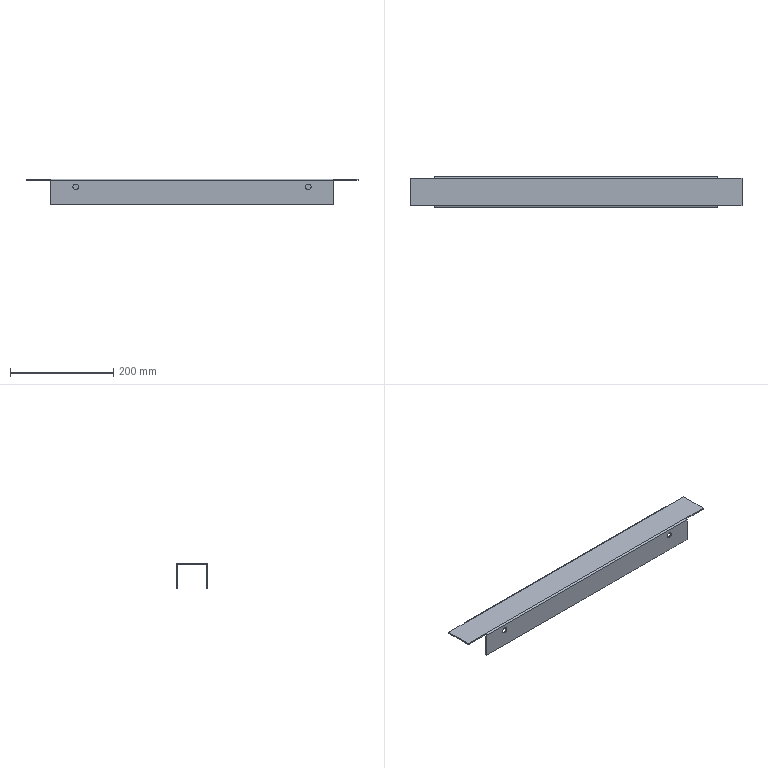Part | SolidWorks | features Cut 2, EdgeFlange 1, FlatPattern 1, ICE 1, MirrorPattern 1, SMBaseFlange 1, SheetMetal 1 | 1 solid | 34 faces | box 644 x 60 x 50 mm | volume 222593 mm3 | plane 22 | cylinder 12 | commonest cylinder face diameters 10.5 x4 11 x4 1 x2 6 x2
STEP:
#1=CARTESIAN_POINT('',(-225.5,-27.5,-9.5));
#2=VERTEX_POINT('',#1);
#3=CARTESIAN_POINT('',(-225.5,-27.5,-20.5));
#4=VERTEX_POINT('',#3);
#5=CARTESIAN_POINT('',(-225.5,-27.5,-15.));
#6=DIRECTION('',(0.,-1.,0.));
#7=DIRECTION('',(0.,0.,1.));
#8=AXIS2_PLACEMENT_3D('',#5,#6,#7);
#9=CIRCLE('',#8,5.5);
#10=EDGE_CURVE('',#2,#4,#9,.T.);
#11=ORIENTED_EDGE('',*,*,#10,.F.);
#12=CARTESIAN_POINT('',(-225.5,-30.,-9.5));
#13=VERTEX_POINT('',#12);
#14=CARTESIAN_POINT('',(-225.5,-20.,-9.5));
#15=DIRECTION('',(0.,-1.,0.));
#16=VECTOR('',#15,1000.);
#17=LINE('',#14,#16);
#18=EDGE_CURVE('',#2,#13,#17,.T.);
#19=ORIENTED_EDGE('',*,*,#18,.T.);
#20=CARTESIAN_POINT('',(-225.5,-30.,-20.5));
#21=VERTEX_POINT('',#20);
#22=CARTESIAN_POINT('',(-225.5,-30.,-15.));
#23=DIRECTION('',(0.,1.,0.));
#24=DIRECTION('',(0.,0.,-1.));
#25=AXIS2_PLACEMENT_3D('',#22,#23,#24);
#26=CIRCLE('',#25,5.5);
#27=EDGE_CURVE('',#21,#13,#26,.T.);
#28=ORIENTED_EDGE('',*,*,#27,.F.);
#29=CARTESIAN_POINT('',(-225.5,-20.,-20.5));
#30=DIRECTION('',(0.,-1.,0.));
#31=VECTOR('',#30,1000.);
#32=LINE('',#29,#31);
#33=EDGE_CURVE('',#4,#21,#32,.T.);
#34=ORIENTED_EDGE('',*,*,#33,.F.);
#35=EDGE_LOOP('',(#11,#19,#28,#34));
#36=FACE_OUTER_BOUND('',#35,.T.);
#37=CARTESIAN_POINT('',(-225.5,-20.,-15.));
#38=DIRECTION('',(0.,-1.,0.));
#39=DIRECTION('',(0.,0.,-1.));
#40=AXIS2_PLACEMENT_3D('',#37,#38,#39);
#41=CYLINDRICAL_SURFACE('',#40,5.5);
#42=ADVANCED_FACE('',(#36),#41,.F.);
#43=CARTESIAN_POINT('',(225.5,-27.5,-20.5));
#44=VERTEX_POINT('',#43);
#45=CARTESIAN_POINT('',(225.5,-27.5,-9.5));
#46=VERTEX_POINT('',#45);
#47=CARTESIAN_POINT('',(225.5,-27.5,-15.));
#48=DIRECTION('',(0.,1.,0.));
#49=DIRECTION('',(0.,0.,1.));
#50=AXIS2_PLACEMENT_3D('',#47,#48,#49);
#51=CIRCLE('',#50,5.5);
#52=EDGE_CURVE('',#44,#46,#51,.T.);
#53=ORIENTED_EDGE('',*,*,#52,.T.);
#54=CARTESIAN_POINT('',(225.5,-30.,-9.5));
#55=VERTEX_POINT('',#54);
#56=CARTESIAN_POINT('',(225.5,-20.,-9.5));
#57=DIRECTION('',(0.,-1.,0.));
#58=VECTOR('',#57,1000.);
#59=LINE('',#56,#58);
#60=EDGE_CURVE('',#46,#55,#59,.T.);
#61=ORIENTED_EDGE('',*,*,#60,.T.);
#62=CARTESIAN_POINT('',(225.5,-30.,-20.5));
#63=VERTEX_POINT('',#62);
#64=CARTESIAN_POINT('',(225.5,-30.,-15.));
#65=DIRECTION('',(0.,-1.,0.));
#66=DIRECTION('',(0.,0.,-1.));
#67=AXIS2_PLACEMENT_3D('',#64,#65,#66);
#68=CIRCLE('',#67,5.5);
#69=EDGE_CURVE('',#55,#63,#68,.T.);
#70=ORIENTED_EDGE('',*,*,#69,.T.);
#71=CARTESIAN_POINT('',(225.5,-20.,-20.5));
#72=DIRECTION('',(0.,-1.,0.));
#73=VECTOR('',#72,1000.);
#74=LINE('',#71,#73);
#75=EDGE_CURVE('',#44,#63,#74,.T.);
#76=ORIENTED_EDGE('',*,*,#75,.F.);
#77=EDGE_LOOP('',(#53,#61,#70,#76));
#78=FACE_OUTER_BOUND('',#77,.T.);
#79=CARTESIAN_POINT('',(225.5,-20.,-15.));
#80=DIRECTION('',(0.,-1.,0.));
#81=DIRECTION('',(0.,0.,-1.));
#82=AXIS2_PLACEMENT_3D('',#79,#80,#81);
#83=CYLINDRICAL_SURFACE('',#82,5.5);
#84=ADVANCED_FACE('',(#78),#83,.F.);
#85=CARTESIAN_POINT('',(225.,27.5,-30.25));
#86=VERTEX_POINT('',#85);
#87=CARTESIAN_POINT('',(225.,27.5,-19.75));
#88=VERTEX_POINT('',#87);
#89=CARTESIAN_POINT('',(225.,27.5,-25.));
#90=DIRECTION('',(0.,1.,0.));
#91=DIRECTION('',(0.,0.,1.));
#92=AXIS2_PLACEMENT_3D('',#89,#90,#91);
#93=CIRCLE('',#92,5.25);
#94=EDGE_CURVE('',#86,#88,#93,.T.);
#95=ORIENTED_EDGE('',*,*,#94,.F.);
#96=CARTESIAN_POINT('',(225.,30.,-30.25));
#97=VERTEX_POINT('',#96);
#98=CARTESIAN_POINT('',(225.,20.,-30.25));
#99=DIRECTION('',(0.,1.,0.));
#100=VECTOR('',#99,1000.);
#101=LINE('',#98,#100);
#102=EDGE_CURVE('',#86,#97,#101,.T.);
#103=ORIENTED_EDGE('',*,*,#102,.T.);
#104=CARTESIAN_POINT('',(225.,30.,-19.75));
#105=VERTEX_POINT('',#104);
#106=CARTESIAN_POINT('',(225.,30.,-25.));
#107=DIRECTION('',(0.,1.,0.));
#108=DIRECTION('',(0.,0.,-1.));
#109=AXIS2_PLACEMENT_3D('',#106,#107,#108);
#110=CIRCLE('',#109,5.25);
#111=EDGE_CURVE('',#97,#105,#110,.T.);
#112=ORIENTED_EDGE('',*,*,#111,.T.);
#113=CARTESIAN_POINT('',(225.,20.,-19.75));
#114=DIRECTION('',(0.,1.,0.));
#115=VECTOR('',#114,1000.);
#116=LINE('',#113,#115);
#117=EDGE_CURVE('',#88,#105,#116,.T.);
#118=ORIENTED_EDGE('',*,*,#117,.F.);
#119=EDGE_LOOP('',(#95,#103,#112,#118));
#120=FACE_OUTER_BOUND('',#119,.T.);
#121=CARTESIAN_POINT('',(225.,20.,-25.));
#122=DIRECTION('',(0.,1.,0.));
#123=DIRECTION('',(0.,0.,1.));
#124=AXIS2_PLACEMENT_3D('',#121,#122,#123);
#125=CYLINDRICAL_SURFACE('',#124,5.25);
#126=ADVANCED_FACE('',(#120),#125,.F.);
#127=CARTESIAN_POINT('',(-225.,27.5,-30.25));
#128=VERTEX_POINT('',#127);
#129=CARTESIAN_POINT('',(-225.,27.5,-19.75));
#130=VERTEX_POINT('',#129);
#131=CARTESIAN_POINT('',(-225.,27.5,-25.));
#132=DIRECTION('',(0.,1.,0.));
#133=DIRECTION('',(0.,0.,1.));
#134=AXIS2_PLACEMENT_3D('',#131,#132,#133);
#135=CIRCLE('',#134,5.25);
#136=EDGE_CURVE('',#128,#130,#135,.T.);
#137=ORIENTED_EDGE('',*,*,#136,.F.);
#138=CARTESIAN_POINT('',(-225.,30.,-30.25));
#139=VERTEX_POINT('',#138);
#140=CARTESIAN_POINT('',(-225.,20.,-30.25));
#141=DIRECTION('',(0.,1.,0.));
#142=VECTOR('',#141,1000.);
#143=LINE('',#140,#142);
#144=EDGE_CURVE('',#128,#139,#143,.T.);
#145=ORIENTED_EDGE('',*,*,#144,.T.);
#146=CARTESIAN_POINT('',(-225.,30.,-19.75));
#147=VERTEX_POINT('',#146);
#148=CARTESIAN_POINT('',(-225.,30.,-25.));
#149=DIRECTION('',(0.,1.,0.));
#150=DIRECTION('',(0.,0.,1.));
#151=AXIS2_PLACEMENT_3D('',#148,#149,#150);
#152=CIRCLE('',#151,5.25);
#153=EDGE_CURVE('',#139,#147,#152,.T.);
#154=ORIENTED_EDGE('',*,*,#153,.T.);
#155=CARTESIAN_POINT('',(-225.,20.,-19.75));
#156=DIRECTION('',(0.,1.,0.));
#157=VECTOR('',#156,1000.);
#158=LINE('',#155,#157);
#159=EDGE_CURVE('',#130,#147,#158,.T.);
#160=ORIENTED_EDGE('',*,*,#159,.F.);
#161=EDGE_LOOP('',(#137,#145,#154,#160));
#162=FACE_OUTER_BOUND('',#161,.T.);
#163=CARTESIAN_POINT('',(-225.,20.,-25.));
#164=DIRECTION('',(0.,1.,0.));
#165=DIRECTION('',(0.,0.,1.));
#166=AXIS2_PLACEMENT_3D('',#163,#164,#165);
#167=CYLINDRICAL_SURFACE('',#166,5.25);
#168=ADVANCED_FACE('',(#162),#167,.F.);
#169=CARTESIAN_POINT('',(-274.5,-30.,-3.));
#170=VERTEX_POINT('',#169);
#171=CARTESIAN_POINT('',(274.5,-30.,-3.));
#172=VERTEX_POINT('',#171);
#173=CARTESIAN_POINT('',(274.5,-30.,-3.));
#174=DIRECTION('',(1.,0.,0.));
#175=VECTOR('',#174,1000.);
#176=LINE('',#173,#175);
#177=EDGE_CURVE('',#170,#172,#176,.T.);
#178=ORIENTED_EDGE('',*,*,#177,.F.);
#179=CARTESIAN_POINT('',(-274.5,-30.,-50.));
#180=VERTEX_POINT('',#179);
#181=CARTESIAN_POINT('',(-274.5,-30.,-50.));
#182=DIRECTION('',(0.,0.,1.));
#183=VECTOR('',#182,1000.);
#184=LINE('',#181,#183);
#185=EDGE_CURVE('',#180,#170,#184,.T.);
#186=ORIENTED_EDGE('',*,*,#185,.F.);
#187=CARTESIAN_POINT('',(274.5,-30.,-50.));
#188=VERTEX_POINT('',#187);
#189=CARTESIAN_POINT('',(274.5,-30.,-50.));
#190=DIRECTION('',(-1.,0.,0.));
#191=VECTOR('',#190,1000.);
#192=LINE('',#189,#191);
#193=EDGE_CURVE('',#188,#180,#192,.T.);
#194=ORIENTED_EDGE('',*,*,#193,.F.);
#195=CARTESIAN_POINT('',(274.5,-30.,-2.5));
#196=DIRECTION('',(0.,0.,-1.));
#197=VECTOR('',#196,1000.);
#198=LINE('',#195,#197);
#199=EDGE_CURVE('',#172,#188,#198,.T.);
#200=ORIENTED_EDGE('',*,*,#199,.F.);
#201=EDGE_LOOP('',(#178,#186,#194,#200));
#202=FACE_OUTER_BOUND('',#201,.T.);
#203=CARTESIAN_POINT('',(225.5,-30.,-15.));
#204=DIRECTION('',(0.,-1.,0.));
#205=DIRECTION('',(0.,0.,-1.));
#206=AXIS2_PLACEMENT_3D('',#203,#204,#205);
#207=CIRCLE('',#206,5.5);
#208=EDGE_CURVE('',#63,#55,#207,.T.);
#209=ORIENTED_EDGE('',*,*,#208,.F.);
#210=ORIENTED_EDGE('',*,*,#69,.F.);
#211=EDGE_LOOP('',(#209,#210));
#212=FACE_BOUND('',#211,.T.);
#213=ORIENTED_EDGE('',*,*,#27,.T.);
#214=CARTESIAN_POINT('',(-225.5,-30.,-15.));
#215=DIRECTION('',(0.,1.,0.));
#216=DIRECTION('',(0.,0.,-1.));
#217=AXIS2_PLACEMENT_3D('',#214,#215,#216);
#218=CIRCLE('',#217,5.5);
#219=EDGE_CURVE('',#13,#21,#218,.T.);
#220=ORIENTED_EDGE('',*,*,#219,.T.);
#221=EDGE_LOOP('',(#213,#220));
#222=FACE_BOUND('',#221,.T.);
#223=CARTESIAN_POINT('',(0.,-30.,0.));
#224=DIRECTION('',(0.,1.,0.));
#225=DIRECTION('',(0.,0.,1.));
#226=AXIS2_PLACEMENT_3D('',#223,#224,#225);
#227=PLANE('',#226);
#228=ADVANCED_FACE('',(#202,#212,#222),#227,.F.);
#229=CARTESIAN_POINT('',(-274.5,-27.5,-50.));
#230=VERTEX_POINT('',#229);
#231=CARTESIAN_POINT('',(-274.5,-27.5,-3.));
#232=VERTEX_POINT('',#231);
#233=CARTESIAN_POINT('',(-274.5,-27.5,0.));
#234=DIRECTION('',(0.,0.,1.));
#235=VECTOR('',#234,1000.);
#236=LINE('',#233,#235);
#237=EDGE_CURVE('',#230,#232,#236,.T.);
#238=ORIENTED_EDGE('',*,*,#237,.T.);
#239=CARTESIAN_POINT('',(274.5,-27.5,-3.));
#240=VERTEX_POINT('',#239);
#241=CARTESIAN_POINT('',(274.5,-27.5,-3.));
#242=DIRECTION('',(-1.,0.,0.));
#243=VECTOR('',#242,1000.);
#244=LINE('',#241,#243);
#245=EDGE_CURVE('',#240,#232,#244,.T.);
#246=ORIENTED_EDGE('',*,*,#245,.F.);
#247=CARTESIAN_POINT('',(274.5,-27.5,-50.));
#248=VERTEX_POINT('',#247);
#249=CARTESIAN_POINT('',(274.5,-27.5,0.));
#250=DIRECTION('',(0.,0.,-1.));
#251=VECTOR('',#250,1000.);
#252=LINE('',#249,#251);
#253=EDGE_CURVE('',#240,#248,#252,.T.);
#254=ORIENTED_EDGE('',*,*,#253,.T.);
#255=CARTESIAN_POINT('',(0.,-27.5,-50.));
#256=DIRECTION('',(-1.,0.,0.));
#257=VECTOR('',#256,1000.);
#258=LINE('',#255,#257);
#259=EDGE_CURVE('',#248,#230,#258,.T.);
#260=ORIENTED_EDGE('',*,*,#259,.T.);
#261=EDGE_LOOP('',(#238,#246,#254,#260));
#262=FACE_OUTER_BOUND('',#261,.T.);
#263=ORIENTED_EDGE('',*,*,#52,.F.);
#264=CARTESIAN_POINT('',(225.5,-27.5,-15.));
#265=DIRECTION('',(0.,1.,0.));
#266=DIRECTION('',(0.,0.,1.));
#267=AXIS2_PLACEMENT_3D('',#264,#265,#266);
#268=CIRCLE('',#267,5.5);
#269=EDGE_CURVE('',#46,#44,#268,.T.);
#270=ORIENTED_EDGE('',*,*,#269,.F.);
#271=EDGE_LOOP('',(#263,#270));
#272=FACE_BOUND('',#271,.T.);
#273=CARTESIAN_POINT('',(-225.5,-27.5,-15.));
#274=DIRECTION('',(0.,-1.,0.));
#275=DIRECTION('',(0.,0.,1.));
#276=AXIS2_PLACEMENT_3D('',#273,#274,#275);
#277=CIRCLE('',#276,5.5);
#278=EDGE_CURVE('',#4,#2,#277,.T.);
#279=ORIENTED_EDGE('',*,*,#278,.T.);
#280=ORIENTED_EDGE('',*,*,#10,.T.);
#281=EDGE_LOOP('',(#279,#280));
#282=FACE_BOUND('',#281,.T.);
#283=CARTESIAN_POINT('',(0.,-27.5,0.));
#284=DIRECTION('',(0.,1.,0.));
#285=DIRECTION('',(0.,0.,1.));
#286=AXIS2_PLACEMENT_3D('',#283,#284,#285);
#287=PLANE('',#286);
#288=ADVANCED_FACE('',(#262,#272,#282),#287,.T.);
#289=CARTESIAN_POINT('',(-322.,-27.,-2.5));
#290=VERTEX_POINT('',#289);
#291=CARTESIAN_POINT('',(-274.5,-27.,-2.5));
#292=VERTEX_POINT('',#291);
#293=CARTESIAN_POINT('',(-322.,-27.,-2.5));
#294=DIRECTION('',(1.,0.,0.));
#295=VECTOR('',#294,1000.);
#296=LINE('',#293,#295);
#297=EDGE_CURVE('',#290,#292,#296,.T.);
#298=ORIENTED_EDGE('',*,*,#297,.T.);
#299=CARTESIAN_POINT('',(-274.5,-27.,0.));
#300=VERTEX_POINT('',#299);
#301=CARTESIAN_POINT('',(-274.5,-27.,-2.5));
#302=DIRECTION('',(0.,0.,1.));
#303=VECTOR('',#302,1000.);
#304=LINE('',#301,#303);
#305=EDGE_CURVE('',#292,#300,#304,.T.);
#306=ORIENTED_EDGE('',*,*,#305,.T.);
#307=CARTESIAN_POINT('',(-322.,-27.,0.));
#308=VERTEX_POINT('',#307);
#309=CARTESIAN_POINT('',(-322.,-27.,0.));
#310=DIRECTION('',(1.,0.,0.));
#311=VECTOR('',#310,1000.);
#312=LINE('',#309,#311);
#313=EDGE_CURVE('',#308,#300,#312,.T.);
#314=ORIENTED_EDGE('',*,*,#313,.F.);
#315=CARTESIAN_POINT('',(-322.,-27.,-2.5));
#316=DIRECTION('',(0.,0.,1.));
#317=VECTOR('',#316,1000.);
#318=LINE('',#315,#317);
#319=EDGE_CURVE('',#290,#308,#318,.T.);
#320=ORIENTED_EDGE('',*,*,#319,.F.);
#321=EDGE_LOOP('',(#298,#306,#314,#320));
#322=FACE_OUTER_BOUND('',#321,.T.);
#323=CARTESIAN_POINT('',(-322.,-27.,-2.5));
#324=DIRECTION('',(0.,-1.,0.));
#325=DIRECTION('',(0.,0.,-1.));
#326=AXIS2_PLACEMENT_3D('',#323,#324,#325);
#327=PLANE('',#326);
#328=ADVANCED_FACE('',(#322),#327,.T.);
#329=CARTESIAN_POINT('',(322.,27.,-2.5));
#330=VERTEX_POINT('',#329);
#331=CARTESIAN_POINT('',(274.5,27.,-2.5));
#332=VERTEX_POINT('',#331);
#333=CARTESIAN_POINT('',(-322.,27.,-2.5));
#334=DIRECTION('',(-1.,0.,0.));
#335=VECTOR('',#334,1000.);
#336=LINE('',#333,#335);
#337=EDGE_CURVE('',#330,#332,#336,.T.);
#338=ORIENTED_EDGE('',*,*,#337,.T.);
#339=CARTESIAN_POINT('',(274.5,27.,0.));
#340=VERTEX_POINT('',#339);
#341=CARTESIAN_POINT('',(274.5,27.,-2.5));
#342=DIRECTION('',(0.,0.,1.));
#343=VECTOR('',#342,1000.);
#344=LINE('',#341,#343);
#345=EDGE_CURVE('',#332,#340,#344,.T.);
#346=ORIENTED_EDGE('',*,*,#345,.T.);
#347=CARTESIAN_POINT('',(322.,27.,0.));
#348=VERTEX_POINT('',#347);
#349=CARTESIAN_POINT('',(-322.,27.,0.));
#350=DIRECTION('',(-1.,0.,0.));
#351=VECTOR('',#350,1000.);
#352=LINE('',#349,#351);
#353=EDGE_CURVE('',#348,#340,#352,.T.);
#354=ORIENTED_EDGE('',*,*,#353,.F.);
#355=CARTESIAN_POINT('',(322.,27.,-2.5));
#356=DIRECTION('',(0.,0.,1.));
#357=VECTOR('',#356,1000.);
#358=LINE('',#355,#357);
#359=EDGE_CURVE('',#330,#348,#358,.T.);
#360=ORIENTED_EDGE('',*,*,#359,.F.);
#361=EDGE_LOOP('',(#338,#346,#354,#360));
#362=FACE_OUTER_BOUND('',#361,.T.);
#363=CARTESIAN_POINT('',(-322.,27.,-2.5));
#364=DIRECTION('',(0.,1.,0.));
#365=DIRECTION('',(0.,0.,1.));
#366=AXIS2_PLACEMENT_3D('',#363,#364,#365);
#367=PLANE('',#366);
#368=ADVANCED_FACE('',(#362),#367,.T.);
#369=CARTESIAN_POINT('',(322.,-27.,0.));
#370=VERTEX_POINT('',#369);
#371=CARTESIAN_POINT('',(322.,27.,0.));
#372=DIRECTION('',(0.,1.,0.));
#373=VECTOR('',#372,1000.);
#374=LINE('',#371,#373);
#375=EDGE_CURVE('',#370,#348,#374,.T.);
#376=ORIENTED_EDGE('',*,*,#375,.F.);
#377=CARTESIAN_POINT('',(322.,-27.,-2.5));
#378=VERTEX_POINT('',#377);
#379=CARTESIAN_POINT('',(322.,-27.,-2.5));
#380=DIRECTION('',(0.,0.,1.));
#381=VECTOR('',#380,1000.);
#382=LINE('',#379,#381);
#383=EDGE_CURVE('',#378,#370,#382,.T.);
#384=ORIENTED_EDGE('',*,*,#383,.F.);
#385=CARTESIAN_POINT('',(322.,27.,-2.5));
#386=DIRECTION('',(0.,1.,0.));
#387=VECTOR('',#386,1000.);
#388=LINE('',#385,#387);
#389=EDGE_CURVE('',#378,#330,#388,.T.);
#390=ORIENTED_EDGE('',*,*,#389,.T.);
#391=ORIENTED_EDGE('',*,*,#359,.T.);
#392=EDGE_LOOP('',(#376,#384,#390,#391));
#393=FACE_OUTER_BOUND('',#392,.T.);
#394=CARTESIAN_POINT('',(322.,27.,-2.5));
#395=DIRECTION('',(1.,0.,0.));
#396=DIRECTION('',(0.,0.,-1.));
#397=AXIS2_PLACEMENT_3D('',#394,#395,#396);
#398=PLANE('',#397);
#399=ADVANCED_FACE('',(#393),#398,.T.);
#400=CARTESIAN_POINT('',(274.5,-27.,-2.5));
#401=VERTEX_POINT('',#400);
#402=CARTESIAN_POINT('',(274.5,-27.,0.));
#403=VERTEX_POINT('',#402);
#404=CARTESIAN_POINT('',(274.5,-27.,-2.5));
#405=DIRECTION('',(0.,0.,1.));
#406=VECTOR('',#405,1000.);
#407=LINE('',#404,#406);
#408=EDGE_CURVE('',#401,#403,#407,.T.);
#409=ORIENTED_EDGE('',*,*,#408,.F.);
#410=CARTESIAN_POINT('',(-322.,-27.,-2.5));
#411=DIRECTION('',(1.,0.,0.));
#412=VECTOR('',#411,1000.);
#413=LINE('',#410,#412);
#414=EDGE_CURVE('',#401,#378,#413,.T.);
#415=ORIENTED_EDGE('',*,*,#414,.T.);
#416=ORIENTED_EDGE('',*,*,#383,.T.);
#417=CARTESIAN_POINT('',(-322.,-27.,0.));
#418=DIRECTION('',(1.,0.,0.));
#419=VECTOR('',#418,1000.);
#420=LINE('',#417,#419);
#421=EDGE_CURVE('',#403,#370,#420,.T.);
#422=ORIENTED_EDGE('',*,*,#421,.F.);
#423=EDGE_LOOP('',(#409,#415,#416,#422));
#424=FACE_OUTER_BOUND('',#423,.T.);
#425=CARTESIAN_POINT('',(-322.,-27.,-2.5));
#426=DIRECTION('',(0.,-1.,0.));
#427=DIRECTION('',(0.,0.,-1.));
#428=AXIS2_PLACEMENT_3D('',#425,#426,#427);
#429=PLANE('',#428);
#430=ADVANCED_FACE('',(#424),#429,.T.);
#431=CARTESIAN_POINT('',(-322.,27.,0.));
#432=VERTEX_POINT('',#431);
#433=CARTESIAN_POINT('',(-322.,27.,0.));
#434=DIRECTION('',(0.,-1.,0.));
#435=VECTOR('',#434,1000.);
#436=LINE('',#433,#435);
#437=EDGE_CURVE('',#432,#308,#436,.T.);
#438=ORIENTED_EDGE('',*,*,#437,.F.);
#439=CARTESIAN_POINT('',(-322.,27.,-2.5));
#440=VERTEX_POINT('',#439);
#441=CARTESIAN_POINT('',(-322.,27.,-2.5));
#442=DIRECTION('',(0.,0.,1.));
#443=VECTOR('',#442,1000.);
#444=LINE('',#441,#443);
#445=EDGE_CURVE('',#440,#432,#444,.T.);
#446=ORIENTED_EDGE('',*,*,#445,.F.);
#447=CARTESIAN_POINT('',(-322.,27.,-2.5));
#448=DIRECTION('',(0.,-1.,0.));
#449=VECTOR('',#448,1000.);
#450=LINE('',#447,#449);
#451=EDGE_CURVE('',#440,#290,#450,.T.);
#452=ORIENTED_EDGE('',*,*,#451,.T.);
#453=ORIENTED_EDGE('',*,*,#319,.T.);
#454=EDGE_LOOP('',(#438,#446,#452,#453));
#455=FACE_OUTER_BOUND('',#454,.T.);
#456=CARTESIAN_POINT('',(-322.,27.,-2.5));
#457=DIRECTION('',(-1.,0.,0.));
#458=DIRECTION('',(0.,0.,1.));
#459=AXIS2_PLACEMENT_3D('',#456,#457,#458);
#460=PLANE('',#459);
#461=ADVANCED_FACE('',(#455),#460,.T.);
#462=CARTESIAN_POINT('',(-274.5,27.,-2.5));
#463=VERTEX_POINT('',#462);
#464=CARTESIAN_POINT('',(-274.5,27.,0.));
#465=VERTEX_POINT('',#464);
#466=CARTESIAN_POINT('',(-274.5,27.,-2.5));
#467=DIRECTION('',(0.,0.,1.));
#468=VECTOR('',#467,1000.);
#469=LINE('',#466,#468);
#470=EDGE_CURVE('',#463,#465,#469,.T.);
#471=ORIENTED_EDGE('',*,*,#470,.F.);
#472=CARTESIAN_POINT('',(-322.,27.,-2.5));
#473=DIRECTION('',(-1.,0.,0.));
#474=VECTOR('',#473,1000.);
#475=LINE('',#472,#474);
#476=EDGE_CURVE('',#463,#440,#475,.T.);
#477=ORIENTED_EDGE('',*,*,#476,.T.);
#478=ORIENTED_EDGE('',*,*,#445,.T.);
#479=CARTESIAN_POINT('',(-322.,27.,0.));
#480=DIRECTION('',(-1.,0.,0.));
#481=VECTOR('',#480,1000.);
#482=LINE('',#479,#481);
#483=EDGE_CURVE('',#465,#432,#482,.T.);
#484=ORIENTED_EDGE('',*,*,#483,.F.);
#485=EDGE_LOOP('',(#471,#477,#478,#484));
#486=FACE_OUTER_BOUND('',#485,.T.);
#487=CARTESIAN_POINT('',(-322.,27.,-2.5));
#488=DIRECTION('',(0.,1.,0.));
#489=DIRECTION('',(0.,0.,1.));
#490=AXIS2_PLACEMENT_3D('',#487,#488,#489);
#491=PLANE('',#490);
#492=ADVANCED_FACE('',(#486),#491,.T.);
#493=ORIENTED_EDGE('',*,*,#389,.F.);
#494=ORIENTED_EDGE('',*,*,#414,.F.);
#495=CARTESIAN_POINT('',(-274.5,-27.,-2.5));
#496=DIRECTION('',(1.,0.,0.));
#497=VECTOR('',#496,1000.);
#498=LINE('',#495,#497);
#499=EDGE_CURVE('',#292,#401,#498,.T.);
#500=ORIENTED_EDGE('',*,*,#499,.F.);
#501=ORIENTED_EDGE('',*,*,#297,.F.);
#502=ORIENTED_EDGE('',*,*,#451,.F.);
#503=ORIENTED_EDGE('',*,*,#476,.F.);
#504=CARTESIAN_POINT('',(274.5,27.,-2.5));
#505=DIRECTION('',(-1.,0.,0.));
#506=VECTOR('',#505,1000.);
#507=LINE('',#504,#506);
#508=EDGE_CURVE('',#332,#463,#507,.T.);
#509=ORIENTED_EDGE('',*,*,#508,.F.);
#510=ORIENTED_EDGE('',*,*,#337,.F.);
#511=EDGE_LOOP('',(#493,#494,#500,#501,#502,#503,#509,#510));
#512=FACE_OUTER_BOUND('',#511,.T.);
#513=CARTESIAN_POINT('',(0.,0.,-2.5));
#514=DIRECTION('',(0.,0.,1.));
#515=DIRECTION('',(1.,0.,0.));
#516=AXIS2_PLACEMENT_3D('',#513,#514,#515);
#517=PLANE('',#516);
#518=ADVANCED_FACE('',(#512),#517,.F.);
#519=ORIENTED_EDGE('',*,*,#375,.T.);
#520=ORIENTED_EDGE('',*,*,#353,.T.);
#521=CARTESIAN_POINT('',(274.5,27.,0.));
#522=DIRECTION('',(-1.,0.,0.));
#523=VECTOR('',#522,1000.);
#524=LINE('',#521,#523);
#525=EDGE_CURVE('',#340,#465,#524,.T.);
#526=ORIENTED_EDGE('',*,*,#525,.T.);
#527=ORIENTED_EDGE('',*,*,#483,.T.);
#528=ORIENTED_EDGE('',*,*,#437,.T.);
#529=ORIENTED_EDGE('',*,*,#313,.T.);
#530=CARTESIAN_POINT('',(-274.5,-27.,0.));
#531=DIRECTION('',(1.,0.,0.));
#532=VECTOR('',#531,1000.);
#533=LINE('',#530,#532);
#534=EDGE_CURVE('',#300,#403,#533,.T.);
#535=ORIENTED_EDGE('',*,*,#534,.T.);
#536=ORIENTED_EDGE('',*,*,#421,.T.);
#537=EDGE_LOOP('',(#519,#520,#526,#527,#528,#529,#535,#536));
#538=FACE_OUTER_BOUND('',#537,.T.);
#539=CARTESIAN_POINT('',(0.,0.,0.));
#540=DIRECTION('',(0.,0.,1.));
#541=DIRECTION('',(1.,0.,0.));
#542=AXIS2_PLACEMENT_3D('',#539,#540,#541);
#543=PLANE('',#542);
#544=ADVANCED_FACE('',(#538),#543,.T.);
#545=CARTESIAN_POINT('',(-274.5,27.5,-3.));
#546=VERTEX_POINT('',#545);
#547=CARTESIAN_POINT('',(-274.5,30.,-3.));
#548=VERTEX_POINT('',#547);
#549=CARTESIAN_POINT('',(-274.5,30.,-3.));
#550=DIRECTION('',(0.,1.,0.));
#551=VECTOR('',#550,1000.);
#552=LINE('',#549,#551);
#553=EDGE_CURVE('',#546,#548,#552,.T.);
#554=ORIENTED_EDGE('',*,*,#553,.F.);
#555=CARTESIAN_POINT('',(-274.5,27.,-3.));
#556=DIRECTION('',(-1.,0.,0.));
#557=DIRECTION('',(0.,0.,-1.));
#558=AXIS2_PLACEMENT_3D('',#555,#556,#557);
#559=CIRCLE('',#558,0.5);
#560=EDGE_CURVE('',#463,#546,#559,.T.);
#561=ORIENTED_EDGE('',*,*,#560,.F.);
#562=ORIENTED_EDGE('',*,*,#470,.T.);
#563=CARTESIAN_POINT('',(-274.5,27.,-3.));
#564=DIRECTION('',(-1.,0.,0.));
#565=DIRECTION('',(0.,0.,-1.));
#566=AXIS2_PLACEMENT_3D('',#563,#564,#565);
#567=CIRCLE('',#566,3.);
#568=EDGE_CURVE('',#465,#548,#567,.T.);
#569=ORIENTED_EDGE('',*,*,#568,.T.);
#570=EDGE_LOOP('',(#554,#561,#562,#569));
#571=FACE_OUTER_BOUND('',#570,.T.);
#572=CARTESIAN_POINT('',(-274.5,27.,-3.));
#573=DIRECTION('',(-1.,0.,0.));
#574=DIRECTION('',(0.,0.,1.));
#575=AXIS2_PLACEMENT_3D('',#572,#573,#574);
#576=PLANE('',#575);
#577=ADVANCED_FACE('',(#571),#576,.T.);
#578=CARTESIAN_POINT('',(274.5,27.5,-3.));
#579=VERTEX_POINT('',#578);
#580=CARTESIAN_POINT('',(274.5,27.,-3.));
#581=DIRECTION('',(1.,0.,0.));
#582=DIRECTION('',(0.,0.,-1.));
#583=AXIS2_PLACEMENT_3D('',#580,#581,#582);
#584=CIRCLE('',#583,0.5);
#585=EDGE_CURVE('',#579,#332,#584,.T.);
#586=ORIENTED_EDGE('',*,*,#585,.F.);
#587=CARTESIAN_POINT('',(274.5,30.,-3.));
#588=VERTEX_POINT('',#587);
#589=CARTESIAN_POINT('',(274.5,27.5,-3.));
#590=DIRECTION('',(0.,1.,0.));
#591=VECTOR('',#590,1000.);
#592=LINE('',#589,#591);
#593=EDGE_CURVE('',#579,#588,#592,.T.);
#594=ORIENTED_EDGE('',*,*,#593,.T.);
#595=CARTESIAN_POINT('',(274.5,27.,-3.));
#596=DIRECTION('',(1.,0.,0.));
#597=DIRECTION('',(0.,0.,-1.));
#598=AXIS2_PLACEMENT_3D('',#595,#596,#597);
#599=CIRCLE('',#598,3.);
#600=EDGE_CURVE('',#588,#340,#599,.T.);
#601=ORIENTED_EDGE('',*,*,#600,.T.);
#602=ORIENTED_EDGE('',*,*,#345,.F.);
#603=EDGE_LOOP('',(#586,#594,#601,#602));
#604=FACE_OUTER_BOUND('',#603,.T.);
#605=CARTESIAN_POINT('',(274.5,27.,-3.));
#606=DIRECTION('',(-1.,0.,0.));
#607=DIRECTION('',(0.,0.,1.));
#608=AXIS2_PLACEMENT_3D('',#605,#606,#607);
#609=PLANE('',#608);
#610=ADVANCED_FACE('',(#604),#609,.F.);
#611=ORIENTED_EDGE('',*,*,#525,.F.);
#612=ORIENTED_EDGE('',*,*,#600,.F.);
#613=CARTESIAN_POINT('',(0.,30.,-3.));
#614=DIRECTION('',(1.,0.,0.));
#615=VECTOR('',#614,1000.);
#616=LINE('',#613,#615);
#617=EDGE_CURVE('',#548,#588,#616,.T.);
#618=ORIENTED_EDGE('',*,*,#617,.F.);
#619=ORIENTED_EDGE('',*,*,#568,.F.);
#620=EDGE_LOOP('',(#611,#612,#618,#619));
#621=FACE_OUTER_BOUND('',#620,.T.);
#622=CARTESIAN_POINT('',(274.5,27.,-3.));
#623=DIRECTION('',(1.,0.,0.));
#624=DIRECTION('',(0.,1.,0.));
#625=AXIS2_PLACEMENT_3D('',#622,#623,#624);
#626=CYLINDRICAL_SURFACE('',#625,3.);
#627=ADVANCED_FACE('',(#621),#626,.T.);
#628=ORIENTED_EDGE('',*,*,#508,.T.);
#629=ORIENTED_EDGE('',*,*,#560,.T.);
#630=CARTESIAN_POINT('',(-274.5,27.5,-3.));
#631=DIRECTION('',(1.,0.,0.));
#632=VECTOR('',#631,1000.);
#633=LINE('',#630,#632);
#634=EDGE_CURVE('',#546,#579,#633,.T.);
#635=ORIENTED_EDGE('',*,*,#634,.T.);
#636=ORIENTED_EDGE('',*,*,#585,.T.);
#637=EDGE_LOOP('',(#628,#629,#635,#636));
#638=FACE_OUTER_BOUND('',#637,.T.);
#639=CARTESIAN_POINT('',(274.5,27.,-3.));
#640=DIRECTION('',(1.,0.,0.));
#641=DIRECTION('',(0.,1.,0.));
#642=AXIS2_PLACEMENT_3D('',#639,#640,#641);
#643=CYLINDRICAL_SURFACE('',#642,0.5);
#644=ADVANCED_FACE('',(#638),#643,.F.);
#645=CARTESIAN_POINT('',(274.5,30.,-50.));
#646=VERTEX_POINT('',#645);
#647=CARTESIAN_POINT('',(274.5,30.,-2.5));
#648=DIRECTION('',(0.,0.,1.));
#649=VECTOR('',#648,1000.);
#650=LINE('',#647,#649);
#651=EDGE_CURVE('',#646,#588,#650,.T.);
#652=ORIENTED_EDGE('',*,*,#651,.T.);
#653=ORIENTED_EDGE('',*,*,#593,.F.);
#654=CARTESIAN_POINT('',(274.5,27.5,-50.));
#655=VERTEX_POINT('',#654);
#656=CARTESIAN_POINT('',(274.5,27.5,0.));
#657=DIRECTION('',(0.,0.,1.));
#658=VECTOR('',#657,1000.);
#659=LINE('',#656,#658);
#660=EDGE_CURVE('',#655,#579,#659,.T.);
#661=ORIENTED_EDGE('',*,*,#660,.F.);
#662=CARTESIAN_POINT('',(274.5,30.,-50.));
#663=DIRECTION('',(0.,-1.,0.));
#664=VECTOR('',#663,1000.);
#665=LINE('',#662,#664);
#666=EDGE_CURVE('',#646,#655,#665,.T.);
#667=ORIENTED_EDGE('',*,*,#666,.F.);
#668=EDGE_LOOP('',(#652,#653,#661,#667));
#669=FACE_OUTER_BOUND('',#668,.T.);
#670=CARTESIAN_POINT('',(274.5,30.,-2.5));
#671=DIRECTION('',(1.,0.,0.));
#672=DIRECTION('',(0.,0.,-1.));
#673=AXIS2_PLACEMENT_3D('',#670,#671,#672);
#674=PLANE('',#673);
#675=ADVANCED_FACE('',(#669),#674,.T.);
#676=CARTESIAN_POINT('',(-274.5,27.5,-50.));
#677=VERTEX_POINT('',#676);
#678=CARTESIAN_POINT('',(-274.5,27.5,0.));
#679=DIRECTION('',(0.,0.,-1.));
#680=VECTOR('',#679,1000.);
#681=LINE('',#678,#680);
#682=EDGE_CURVE('',#546,#677,#681,.T.);
#683=ORIENTED_EDGE('',*,*,#682,.F.);
#684=ORIENTED_EDGE('',*,*,#553,.T.);
#685=CARTESIAN_POINT('',(-274.5,30.,-50.));
#686=VERTEX_POINT('',#685);
#687=CARTESIAN_POINT('',(-274.5,30.,-50.));
#688=DIRECTION('',(0.,0.,-1.));
#689=VECTOR('',#688,1000.);
#690=LINE('',#687,#689);
#691=EDGE_CURVE('',#548,#686,#690,.T.);
#692=ORIENTED_EDGE('',*,*,#691,.T.);
#693=CARTESIAN_POINT('',(-274.5,30.,-50.));
#694=DIRECTION('',(0.,-1.,0.));
#695=VECTOR('',#694,1000.);
#696=LINE('',#693,#695);
#697=EDGE_CURVE('',#686,#677,#696,.T.);
#698=ORIENTED_EDGE('',*,*,#697,.T.);
#699=EDGE_LOOP('',(#683,#684,#692,#698));
#700=FACE_OUTER_BOUND('',#699,.T.);
#701=CARTESIAN_POINT('',(-274.5,30.,-50.));
#702=DIRECTION('',(-1.,0.,0.));
#703=DIRECTION('',(0.,0.,1.));
#704=AXIS2_PLACEMENT_3D('',#701,#702,#703);
#705=PLANE('',#704);
#706=ADVANCED_FACE('',(#700),#705,.T.);
#707=CARTESIAN_POINT('',(225.,30.,-25.));
#708=DIRECTION('',(0.,1.,0.));
#709=DIRECTION('',(0.,0.,-1.));
#710=AXIS2_PLACEMENT_3D('',#707,#708,#709);
#711=CIRCLE('',#710,5.25);
#712=EDGE_CURVE('',#105,#97,#711,.T.);
#713=ORIENTED_EDGE('',*,*,#712,.F.);
#714=ORIENTED_EDGE('',*,*,#111,.F.);
#715=EDGE_LOOP('',(#713,#714));
#716=FACE_BOUND('',#715,.T.);
#717=CARTESIAN_POINT('',(-225.,30.,-25.));
#718=DIRECTION('',(0.,1.,0.));
#719=DIRECTION('',(0.,0.,1.));
#720=AXIS2_PLACEMENT_3D('',#717,#718,#719);
#721=CIRCLE('',#720,5.25);
#722=EDGE_CURVE('',#147,#139,#721,.T.);
#723=ORIENTED_EDGE('',*,*,#722,.F.);
#724=ORIENTED_EDGE('',*,*,#153,.F.);
#725=EDGE_LOOP('',(#723,#724));
#726=FACE_BOUND('',#725,.T.);
#727=ORIENTED_EDGE('',*,*,#691,.F.);
#728=ORIENTED_EDGE('',*,*,#617,.T.);
#729=ORIENTED_EDGE('',*,*,#651,.F.);
#730=CARTESIAN_POINT('',(274.5,30.,-50.));
#731=DIRECTION('',(1.,0.,0.));
#732=VECTOR('',#731,1000.);
#733=LINE('',#730,#732);
#734=EDGE_CURVE('',#686,#646,#733,.T.);
#735=ORIENTED_EDGE('',*,*,#734,.F.);
#736=EDGE_LOOP('',(#727,#728,#729,#735));
#737=FACE_OUTER_BOUND('',#736,.T.);
#738=CARTESIAN_POINT('',(0.,30.,0.));
#739=DIRECTION('',(0.,1.,0.));
#740=DIRECTION('',(0.,0.,1.));
#741=AXIS2_PLACEMENT_3D('',#738,#739,#740);
#742=PLANE('',#741);
#743=ADVANCED_FACE('',(#716,#726,#737),#742,.T.);
#744=CARTESIAN_POINT('',(225.,27.5,-25.));
#745=DIRECTION('',(0.,1.,0.));
#746=DIRECTION('',(0.,0.,1.));
#747=AXIS2_PLACEMENT_3D('',#744,#745,#746);
#748=CIRCLE('',#747,5.25);
#749=EDGE_CURVE('',#88,#86,#748,.T.);
#750=ORIENTED_EDGE('',*,*,#749,.T.);
#751=ORIENTED_EDGE('',*,*,#94,.T.);
#752=EDGE_LOOP('',(#750,#751));
#753=FACE_BOUND('',#752,.T.);
#754=CARTESIAN_POINT('',(-225.,27.5,-25.));
#755=DIRECTION('',(0.,1.,0.));
#756=DIRECTION('',(0.,0.,1.));
#757=AXIS2_PLACEMENT_3D('',#754,#755,#756);
#758=CIRCLE('',#757,5.25);
#759=EDGE_CURVE('',#130,#128,#758,.T.);
#760=ORIENTED_EDGE('',*,*,#759,.T.);
#761=ORIENTED_EDGE('',*,*,#136,.T.);
#762=EDGE_LOOP('',(#760,#761));
#763=FACE_BOUND('',#762,.T.);
#764=ORIENTED_EDGE('',*,*,#634,.F.);
#765=ORIENTED_EDGE('',*,*,#682,.T.);
#766=CARTESIAN_POINT('',(0.,27.5,-50.));
#767=DIRECTION('',(1.,0.,0.));
#768=VECTOR('',#767,1000.);
#769=LINE('',#766,#768);
#770=EDGE_CURVE('',#677,#655,#769,.T.);
#771=ORIENTED_EDGE('',*,*,#770,.T.);
#772=ORIENTED_EDGE('',*,*,#660,.T.);
#773=EDGE_LOOP('',(#764,#765,#771,#772));
#774=FACE_OUTER_BOUND('',#773,.T.);
#775=CARTESIAN_POINT('',(0.,27.5,0.));
#776=DIRECTION('',(0.,1.,0.));
#777=DIRECTION('',(0.,0.,1.));
#778=AXIS2_PLACEMENT_3D('',#775,#776,#777);
#779=PLANE('',#778);
#780=ADVANCED_FACE('',(#753,#763,#774),#779,.F.);
#781=ORIENTED_EDGE('',*,*,#770,.F.);
#782=ORIENTED_EDGE('',*,*,#697,.F.);
#783=ORIENTED_EDGE('',*,*,#734,.T.);
#784=ORIENTED_EDGE('',*,*,#666,.T.);
#785=EDGE_LOOP('',(#781,#782,#783,#784));
#786=FACE_OUTER_BOUND('',#785,.T.);
#787=CARTESIAN_POINT('',(274.5,30.,-50.));
#788=DIRECTION('',(0.,0.,-1.));
#789=DIRECTION('',(0.,1.,0.));
#790=AXIS2_PLACEMENT_3D('',#787,#788,#789);
#791=PLANE('',#790);
#792=ADVANCED_FACE('',(#786),#791,.T.);
#793=CARTESIAN_POINT('',(274.5,-30.,-3.));
#794=DIRECTION('',(0.,-1.,0.));
#795=VECTOR('',#794,1000.);
#796=LINE('',#793,#795);
#797=EDGE_CURVE('',#240,#172,#796,.T.);
#798=ORIENTED_EDGE('',*,*,#797,.F.);
#799=CARTESIAN_POINT('',(274.5,-27.,-3.));
#800=DIRECTION('',(1.,0.,0.));
#801=DIRECTION('',(0.,0.,1.));
#802=AXIS2_PLACEMENT_3D('',#799,#800,#801);
#803=CIRCLE('',#802,0.5);
#804=EDGE_CURVE('',#401,#240,#803,.T.);
#805=ORIENTED_EDGE('',*,*,#804,.F.);
#806=ORIENTED_EDGE('',*,*,#408,.T.);
#807=CARTESIAN_POINT('',(274.5,-27.,-3.));
#808=DIRECTION('',(1.,0.,0.));
#809=DIRECTION('',(0.,0.,1.));
#810=AXIS2_PLACEMENT_3D('',#807,#808,#809);
#811=CIRCLE('',#810,3.);
#812=EDGE_CURVE('',#403,#172,#811,.T.);
#813=ORIENTED_EDGE('',*,*,#812,.T.);
#814=EDGE_LOOP('',(#798,#805,#806,#813));
#815=FACE_OUTER_BOUND('',#814,.T.);
#816=CARTESIAN_POINT('',(274.5,-27.,-3.));
#817=DIRECTION('',(1.,0.,0.));
#818=DIRECTION('',(0.,0.,-1.));
#819=AXIS2_PLACEMENT_3D('',#816,#817,#818);
#820=PLANE('',#819);
#821=ADVANCED_FACE('',(#815),#820,.T.);
#822=CARTESIAN_POINT('',(-274.5,-27.,-3.));
#823=DIRECTION('',(-1.,0.,0.));
#824=DIRECTION('',(0.,0.,1.));
#825=AXIS2_PLACEMENT_3D('',#822,#823,#824);
#826=CIRCLE('',#825,0.5);
#827=EDGE_CURVE('',#232,#292,#826,.T.);
#828=ORIENTED_EDGE('',*,*,#827,.F.);
#829=CARTESIAN_POINT('',(-274.5,-27.5,-3.));
#830=DIRECTION('',(0.,-1.,0.));
#831=VECTOR('',#830,1000.);
#832=LINE('',#829,#831);
#833=EDGE_CURVE('',#232,#170,#832,.T.);
#834=ORIENTED_EDGE('',*,*,#833,.T.);
#835=CARTESIAN_POINT('',(-274.5,-27.,-3.));
#836=DIRECTION('',(-1.,0.,0.));
#837=DIRECTION('',(0.,0.,1.));
#838=AXIS2_PLACEMENT_3D('',#835,#836,#837);
#839=CIRCLE('',#838,3.);
#840=EDGE_CURVE('',#170,#300,#839,.T.);
#841=ORIENTED_EDGE('',*,*,#840,.T.);
#842=ORIENTED_EDGE('',*,*,#305,.F.);
#843=EDGE_LOOP('',(#828,#834,#841,#842));
#844=FACE_OUTER_BOUND('',#843,.T.);
#845=CARTESIAN_POINT('',(-274.5,-27.,-3.));
#846=DIRECTION('',(1.,0.,0.));
#847=DIRECTION('',(0.,0.,-1.));
#848=AXIS2_PLACEMENT_3D('',#845,#846,#847);
#849=PLANE('',#848);
#850=ADVANCED_FACE('',(#844),#849,.F.);
#851=ORIENTED_EDGE('',*,*,#534,.F.);
#852=ORIENTED_EDGE('',*,*,#840,.F.);
#853=ORIENTED_EDGE('',*,*,#177,.T.);
#854=ORIENTED_EDGE('',*,*,#812,.F.);
#855=EDGE_LOOP('',(#851,#852,#853,#854));
#856=FACE_OUTER_BOUND('',#855,.T.);
#857=CARTESIAN_POINT('',(-274.5,-27.,-3.));
#858=DIRECTION('',(-1.,0.,0.));
#859=DIRECTION('',(0.,-1.,0.));
#860=AXIS2_PLACEMENT_3D('',#857,#858,#859);
#861=CYLINDRICAL_SURFACE('',#860,3.);
#862=ADVANCED_FACE('',(#856),#861,.T.);
#863=ORIENTED_EDGE('',*,*,#499,.T.);
#864=ORIENTED_EDGE('',*,*,#804,.T.);
#865=ORIENTED_EDGE('',*,*,#245,.T.);
#866=ORIENTED_EDGE('',*,*,#827,.T.);
#867=EDGE_LOOP('',(#863,#864,#865,#866));
#868=FACE_OUTER_BOUND('',#867,.T.);
#869=CARTESIAN_POINT('',(-274.5,-27.,-3.));
#870=DIRECTION('',(-1.,0.,0.));
#871=DIRECTION('',(0.,-1.,0.));
#872=AXIS2_PLACEMENT_3D('',#869,#870,#871);
#873=CYLINDRICAL_SURFACE('',#872,0.5);
#874=ADVANCED_FACE('',(#868),#873,.F.);
#875=ORIENTED_EDGE('',*,*,#253,.F.);
#876=ORIENTED_EDGE('',*,*,#797,.T.);
#877=ORIENTED_EDGE('',*,*,#199,.T.);
#878=CARTESIAN_POINT('',(274.5,-30.,-50.));
#879=DIRECTION('',(0.,1.,0.));
#880=VECTOR('',#879,1000.);
#881=LINE('',#878,#880);
#882=EDGE_CURVE('',#188,#248,#881,.T.);
#883=ORIENTED_EDGE('',*,*,#882,.T.);
#884=EDGE_LOOP('',(#875,#876,#877,#883));
#885=FACE_OUTER_BOUND('',#884,.T.);
#886=CARTESIAN_POINT('',(274.5,-30.,-2.5));
#887=DIRECTION('',(1.,0.,0.));
#888=DIRECTION('',(0.,0.,-1.));
#889=AXIS2_PLACEMENT_3D('',#886,#887,#888);
#890=PLANE('',#889);
#891=ADVANCED_FACE('',(#885),#890,.T.);
#892=ORIENTED_EDGE('',*,*,#185,.T.);
#893=ORIENTED_EDGE('',*,*,#833,.F.);
#894=ORIENTED_EDGE('',*,*,#237,.F.);
#895=CARTESIAN_POINT('',(-274.5,-30.,-50.));
#896=DIRECTION('',(0.,1.,0.));
#897=VECTOR('',#896,1000.);
#898=LINE('',#895,#897);
#899=EDGE_CURVE('',#180,#230,#898,.T.);
#900=ORIENTED_EDGE('',*,*,#899,.F.);
#901=EDGE_LOOP('',(#892,#893,#894,#900));
#902=FACE_OUTER_BOUND('',#901,.T.);
#903=CARTESIAN_POINT('',(-274.5,-30.,-50.));
#904=DIRECTION('',(-1.,0.,0.));
#905=DIRECTION('',(0.,0.,1.));
#906=AXIS2_PLACEMENT_3D('',#903,#904,#905);
#907=PLANE('',#906);
#908=ADVANCED_FACE('',(#902),#907,.T.);
#909=ORIENTED_EDGE('',*,*,#259,.F.);
#910=ORIENTED_EDGE('',*,*,#882,.F.);
#911=ORIENTED_EDGE('',*,*,#193,.T.);
#912=ORIENTED_EDGE('',*,*,#899,.T.);
#913=EDGE_LOOP('',(#909,#910,#911,#912));
#914=FACE_OUTER_BOUND('',#913,.T.);
#915=CARTESIAN_POINT('',(274.5,-30.,-50.));
#916=DIRECTION('',(0.,0.,-1.));
#917=DIRECTION('',(0.,1.,0.));
#918=AXIS2_PLACEMENT_3D('',#915,#916,#917);
#919=PLANE('',#918);
#920=ADVANCED_FACE('',(#914),#919,.T.);
#921=ORIENTED_EDGE('',*,*,#144,.F.);
#922=ORIENTED_EDGE('',*,*,#759,.F.);
#923=ORIENTED_EDGE('',*,*,#159,.T.);
#924=ORIENTED_EDGE('',*,*,#722,.T.);
#925=EDGE_LOOP('',(#921,#922,#923,#924));
#926=FACE_OUTER_BOUND('',#925,.T.);
#927=CARTESIAN_POINT('',(-225.,20.,-25.));
#928=DIRECTION('',(0.,1.,0.));
#929=DIRECTION('',(0.,0.,1.));
#930=AXIS2_PLACEMENT_3D('',#927,#928,#929);
#931=CYLINDRICAL_SURFACE('',#930,5.25);
#932=ADVANCED_FACE('',(#926),#931,.F.);
#933=ORIENTED_EDGE('',*,*,#102,.F.);
#934=ORIENTED_EDGE('',*,*,#749,.F.);
#935=ORIENTED_EDGE('',*,*,#117,.T.);
#936=ORIENTED_EDGE('',*,*,#712,.T.);
#937=EDGE_LOOP('',(#933,#934,#935,#936));
#938=FACE_OUTER_BOUND('',#937,.T.);
#939=CARTESIAN_POINT('',(225.,20.,-25.));
#940=DIRECTION('',(0.,1.,0.));
#941=DIRECTION('',(0.,0.,1.));
#942=AXIS2_PLACEMENT_3D('',#939,#940,#941);
#943=CYLINDRICAL_SURFACE('',#942,5.25);
#944=ADVANCED_FACE('',(#938),#943,.F.);
#945=ORIENTED_EDGE('',*,*,#60,.F.);
#946=ORIENTED_EDGE('',*,*,#269,.T.);
#947=ORIENTED_EDGE('',*,*,#75,.T.);
#948=ORIENTED_EDGE('',*,*,#208,.T.);
#949=EDGE_LOOP('',(#945,#946,#947,#948));
#950=FACE_OUTER_BOUND('',#949,.T.);
#951=CARTESIAN_POINT('',(225.5,-20.,-15.));
#952=DIRECTION('',(0.,-1.,0.));
#953=DIRECTION('',(0.,0.,-1.));
#954=AXIS2_PLACEMENT_3D('',#951,#952,#953);
#955=CYLINDRICAL_SURFACE('',#954,5.5);
#956=ADVANCED_FACE('',(#950),#955,.F.);
#957=ORIENTED_EDGE('',*,*,#18,.F.);
#958=ORIENTED_EDGE('',*,*,#278,.F.);
#959=ORIENTED_EDGE('',*,*,#33,.T.);
#960=ORIENTED_EDGE('',*,*,#219,.F.);
#961=EDGE_LOOP('',(#957,#958,#959,#960));
#962=FACE_OUTER_BOUND('',#961,.T.);
#963=CARTESIAN_POINT('',(-225.5,-20.,-15.));
#964=DIRECTION('',(0.,-1.,0.));
#965=DIRECTION('',(0.,0.,-1.));
#966=AXIS2_PLACEMENT_3D('',#963,#964,#965);
#967=CYLINDRICAL_SURFACE('',#966,5.5);
#968=ADVANCED_FACE('',(#962),#967,.F.);
#969=CLOSED_SHELL('',(#42,#84,#126,#168,#228,#288,#328,#368,#399,#430,#461,#492,#518,#544,#577,#610,#627,#644,#675,#706,#743,#780,#792,#821,#850,#862,#874,#891,#908,#920,#932,#944,#956,#968));
#970=MANIFOLD_SOLID_BREP('',#969);
#971=CARTESIAN_POINT('',(0.,0.,0.));
#972=DIRECTION('',(0.,0.,1.));
#973=DIRECTION('',(1.,0.,0.));
#974=AXIS2_PLACEMENT_3D('',#971,#972,#973);
#975=(LENGTH_UNIT()NAMED_UNIT(*)SI_UNIT(.MILLI.,.METRE.));
#976=UNCERTAINTY_MEASURE_WITH_UNIT(LENGTH_MEASURE(0.00001),#975,'','');
#977=(NAMED_UNIT(*)PLANE_ANGLE_UNIT()SI_UNIT($,.RADIAN.));
#978=(NAMED_UNIT(*)SI_UNIT($,.STERADIAN.)SOLID_ANGLE_UNIT());
#979=(GEOMETRIC_REPRESENTATION_CONTEXT(3)GLOBAL_UNCERTAINTY_ASSIGNED_CONTEXT((#976))GLOBAL_UNIT_ASSIGNED_CONTEXT((#975,#977,#978))REPRESENTATION_CONTEXT('',''));
#980=ADVANCED_BREP_SHAPE_REPRESENTATION('',(#970,#974),#979);